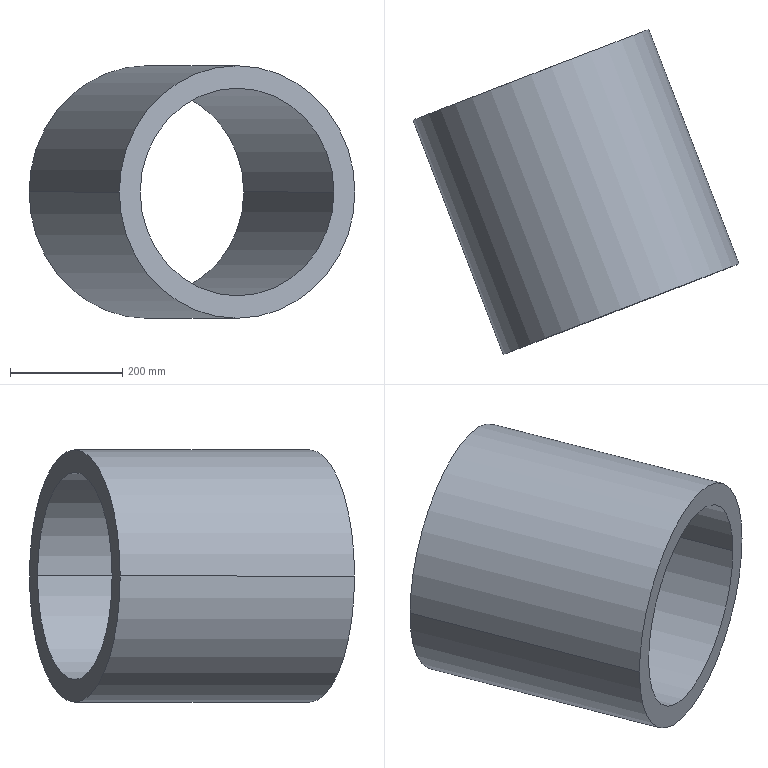Part | SolidWorks | features ICE 2, BaseBody 1, Scale 1 | 1 solid | 6 faces | box 580.701 x 579.323 x 450 mm | volume 23061301 mm3 | cylinder 4 | plane 2 | commonest cylinder face diameters 370 x2 450 x2
STEP:
#1=CARTESIAN_POINT('',(194.57,-303.913,89.5));
#2=VERTEX_POINT('',#1);
#3=CARTESIAN_POINT('',(539.9,-171.068,89.5));
#4=VERTEX_POINT('',#3);
#5=CARTESIAN_POINT('',(367.235,-237.491,89.5));
#6=DIRECTION('',(0.359,-0.9333,-0.000000657));
#7=DIRECTION('',(0.9333,0.359,0.));
#8=AXIS2_PLACEMENT_3D('',#5,#6,#7);
#9=CIRCLE('',#8,185.);
#10=EDGE_CURVE('',#2,#4,#9,.T.);
#11=ORIENTED_EDGE('',*,*,#10,.F.);
#12=CARTESIAN_POINT('',(355.277,-721.668,89.5));
#13=VERTEX_POINT('',#12);
#14=CARTESIAN_POINT('',(140.429,-163.173,89.501));
#15=DIRECTION('',(0.359,-0.9333,-0.000000657));
#16=VECTOR('',#15,1000.);
#17=LINE('',#14,#16);
#18=EDGE_CURVE('',#2,#13,#17,.T.);
#19=ORIENTED_EDGE('',*,*,#18,.T.);
#20=CARTESIAN_POINT('',(700.606,-588.823,89.5));
#21=VERTEX_POINT('',#20);
#22=CARTESIAN_POINT('',(527.941,-655.246,89.5));
#23=DIRECTION('',(0.359,-0.9333,-0.000000657));
#24=DIRECTION('',(0.9333,0.359,0.));
#25=AXIS2_PLACEMENT_3D('',#22,#23,#24);
#26=CIRCLE('',#25,185.);
#27=EDGE_CURVE('',#13,#21,#26,.T.);
#28=ORIENTED_EDGE('',*,*,#27,.T.);
#29=CARTESIAN_POINT('',(485.758,-30.328,89.501));
#30=DIRECTION('',(0.359,-0.9333,-0.000000657));
#31=VECTOR('',#30,1000.);
#32=LINE('',#29,#31);
#33=EDGE_CURVE('',#4,#21,#32,.T.);
#34=ORIENTED_EDGE('',*,*,#33,.F.);
#35=EDGE_LOOP('',(#11,#19,#28,#34));
#36=FACE_OUTER_BOUND('',#35,.T.);
#37=CARTESIAN_POINT('',(313.093,-96.75,89.501));
#38=DIRECTION('',(0.359,-0.9333,-0.000000657));
#39=DIRECTION('',(0.9333,0.359,0.));
#40=AXIS2_PLACEMENT_3D('',#37,#38,#39);
#41=CYLINDRICAL_SURFACE('',#40,185.);
#42=ADVANCED_FACE('',(#36),#41,.F.);
#43=CARTESIAN_POINT('',(157.238,-318.275,89.5));
#44=VERTEX_POINT('',#43);
#45=CARTESIAN_POINT('',(577.232,-156.707,89.5));
#46=VERTEX_POINT('',#45);
#47=CARTESIAN_POINT('',(367.235,-237.491,89.5));
#48=DIRECTION('',(-0.359,0.9333,0.000000657));
#49=DIRECTION('',(0.9333,0.359,0.));
#50=AXIS2_PLACEMENT_3D('',#47,#48,#49);
#51=CIRCLE('',#50,225.);
#52=EDGE_CURVE('',#44,#46,#51,.T.);
#53=ORIENTED_EDGE('',*,*,#52,.F.);
#54=CARTESIAN_POINT('',(317.944,-736.03,89.5));
#55=VERTEX_POINT('',#54);
#56=CARTESIAN_POINT('',(-71.254,275.688,89.501));
#57=DIRECTION('',(0.359,-0.9333,-0.000000657));
#58=VECTOR('',#57,1000.);
#59=LINE('',#56,#58);
#60=EDGE_CURVE('',#44,#55,#59,.T.);
#61=ORIENTED_EDGE('',*,*,#60,.T.);
#62=CARTESIAN_POINT('',(737.939,-574.462,89.5));
#63=VERTEX_POINT('',#62);
#64=CARTESIAN_POINT('',(527.941,-655.246,89.5));
#65=DIRECTION('',(0.359,-0.9333,-0.000000657));
#66=DIRECTION('',(0.9333,0.359,0.));
#67=AXIS2_PLACEMENT_3D('',#64,#65,#66);
#68=CIRCLE('',#67,225.);
#69=EDGE_CURVE('',#63,#55,#68,.T.);
#70=ORIENTED_EDGE('',*,*,#69,.F.);
#71=CARTESIAN_POINT('',(348.741,437.256,89.501));
#72=DIRECTION('',(0.359,-0.9333,-0.000000657));
#73=VECTOR('',#72,1000.);
#74=LINE('',#71,#73);
#75=EDGE_CURVE('',#46,#63,#74,.T.);
#76=ORIENTED_EDGE('',*,*,#75,.F.);
#77=EDGE_LOOP('',(#53,#61,#70,#76));
#78=FACE_OUTER_BOUND('',#77,.T.);
#79=CARTESIAN_POINT('',(138.743,356.472,89.501));
#80=DIRECTION('',(0.359,-0.9333,-0.000000657));
#81=DIRECTION('',(0.9333,0.359,0.));
#82=AXIS2_PLACEMENT_3D('',#79,#80,#81);
#83=CYLINDRICAL_SURFACE('',#82,225.);
#84=ADVANCED_FACE('',(#78),#83,.T.);
#85=ORIENTED_EDGE('',*,*,#60,.F.);
#86=CARTESIAN_POINT('',(367.235,-237.491,89.5));
#87=DIRECTION('',(-0.359,0.9333,0.000000657));
#88=DIRECTION('',(0.9333,0.359,0.));
#89=AXIS2_PLACEMENT_3D('',#86,#87,#88);
#90=CIRCLE('',#89,225.);
#91=EDGE_CURVE('',#46,#44,#90,.T.);
#92=ORIENTED_EDGE('',*,*,#91,.F.);
#93=ORIENTED_EDGE('',*,*,#75,.T.);
#94=CARTESIAN_POINT('',(527.941,-655.246,89.5));
#95=DIRECTION('',(0.359,-0.9333,-0.000000657));
#96=DIRECTION('',(0.9333,0.359,0.));
#97=AXIS2_PLACEMENT_3D('',#94,#95,#96);
#98=CIRCLE('',#97,225.);
#99=EDGE_CURVE('',#55,#63,#98,.T.);
#100=ORIENTED_EDGE('',*,*,#99,.F.);
#101=EDGE_LOOP('',(#85,#92,#93,#100));
#102=FACE_OUTER_BOUND('',#101,.T.);
#103=CARTESIAN_POINT('',(138.743,356.472,89.501));
#104=DIRECTION('',(0.359,-0.9333,-0.000000657));
#105=DIRECTION('',(0.9333,0.359,0.));
#106=AXIS2_PLACEMENT_3D('',#103,#104,#105);
#107=CYLINDRICAL_SURFACE('',#106,225.);
#108=ADVANCED_FACE('',(#102),#107,.T.);
#109=CARTESIAN_POINT('',(367.235,-237.491,89.5));
#110=DIRECTION('',(0.359,-0.9333,-0.000000657));
#111=DIRECTION('',(0.9333,0.359,0.));
#112=AXIS2_PLACEMENT_3D('',#109,#110,#111);
#113=CIRCLE('',#112,185.);
#114=EDGE_CURVE('',#4,#2,#113,.T.);
#115=ORIENTED_EDGE('',*,*,#114,.T.);
#116=ORIENTED_EDGE('',*,*,#10,.T.);
#117=EDGE_LOOP('',(#115,#116));
#118=FACE_BOUND('',#117,.T.);
#119=ORIENTED_EDGE('',*,*,#91,.T.);
#120=ORIENTED_EDGE('',*,*,#52,.T.);
#121=EDGE_LOOP('',(#119,#120));
#122=FACE_OUTER_BOUND('',#121,.T.);
#123=CARTESIAN_POINT('',(367.235,-237.49,-78.5));
#124=DIRECTION('',(0.359,-0.9333,-0.000000657));
#125=DIRECTION('',(0.9333,0.359,0.));
#126=AXIS2_PLACEMENT_3D('',#123,#124,#125);
#127=PLANE('',#126);
#128=ADVANCED_FACE('',(#118,#122),#127,.F.);
#129=CARTESIAN_POINT('',(527.941,-655.246,89.5));
#130=DIRECTION('',(0.359,-0.9333,-0.000000657));
#131=DIRECTION('',(0.9333,0.359,0.));
#132=AXIS2_PLACEMENT_3D('',#129,#130,#131);
#133=CIRCLE('',#132,185.);
#134=EDGE_CURVE('',#21,#13,#133,.T.);
#135=ORIENTED_EDGE('',*,*,#134,.F.);
#136=ORIENTED_EDGE('',*,*,#27,.F.);
#137=EDGE_LOOP('',(#135,#136));
#138=FACE_BOUND('',#137,.T.);
#139=ORIENTED_EDGE('',*,*,#69,.T.);
#140=ORIENTED_EDGE('',*,*,#99,.T.);
#141=EDGE_LOOP('',(#139,#140));
#142=FACE_OUTER_BOUND('',#141,.T.);
#143=CARTESIAN_POINT('',(334.733,-729.571,-120.349));
#144=DIRECTION('',(-0.359,0.9333,0.000000657));
#145=DIRECTION('',(-0.9333,-0.359,0.));
#146=AXIS2_PLACEMENT_3D('',#143,#144,#145);
#147=PLANE('',#146);
#148=ADVANCED_FACE('',(#138,#142),#147,.F.);
#149=ORIENTED_EDGE('',*,*,#18,.F.);
#150=ORIENTED_EDGE('',*,*,#114,.F.);
#151=ORIENTED_EDGE('',*,*,#33,.T.);
#152=ORIENTED_EDGE('',*,*,#134,.T.);
#153=EDGE_LOOP('',(#149,#150,#151,#152));
#154=FACE_OUTER_BOUND('',#153,.T.);
#155=CARTESIAN_POINT('',(313.093,-96.75,89.501));
#156=DIRECTION('',(0.359,-0.9333,-0.000000657));
#157=DIRECTION('',(0.9333,0.359,0.));
#158=AXIS2_PLACEMENT_3D('',#155,#156,#157);
#159=CYLINDRICAL_SURFACE('',#158,185.);
#160=ADVANCED_FACE('',(#154),#159,.F.);
#161=CLOSED_SHELL('',(#42,#84,#108,#128,#148,#160));
#162=MANIFOLD_SOLID_BREP('',#161);
#163=CARTESIAN_POINT('',(0.,0.,0.));
#164=DIRECTION('',(0.,0.,1.));
#165=DIRECTION('',(1.,0.,0.));
#166=AXIS2_PLACEMENT_3D('',#163,#164,#165);
#167=(LENGTH_UNIT()NAMED_UNIT(*)SI_UNIT(.MILLI.,.METRE.));
#168=UNCERTAINTY_MEASURE_WITH_UNIT(LENGTH_MEASURE(0.00001),#167,'','');
#169=(NAMED_UNIT(*)PLANE_ANGLE_UNIT()SI_UNIT($,.RADIAN.));
#170=(NAMED_UNIT(*)SI_UNIT($,.STERADIAN.)SOLID_ANGLE_UNIT());
#171=(GEOMETRIC_REPRESENTATION_CONTEXT(3)GLOBAL_UNCERTAINTY_ASSIGNED_CONTEXT((#168))GLOBAL_UNIT_ASSIGNED_CONTEXT((#167,#169,#170))REPRESENTATION_CONTEXT('',''));
#172=ADVANCED_BREP_SHAPE_REPRESENTATION('',(#162,#166),#171);